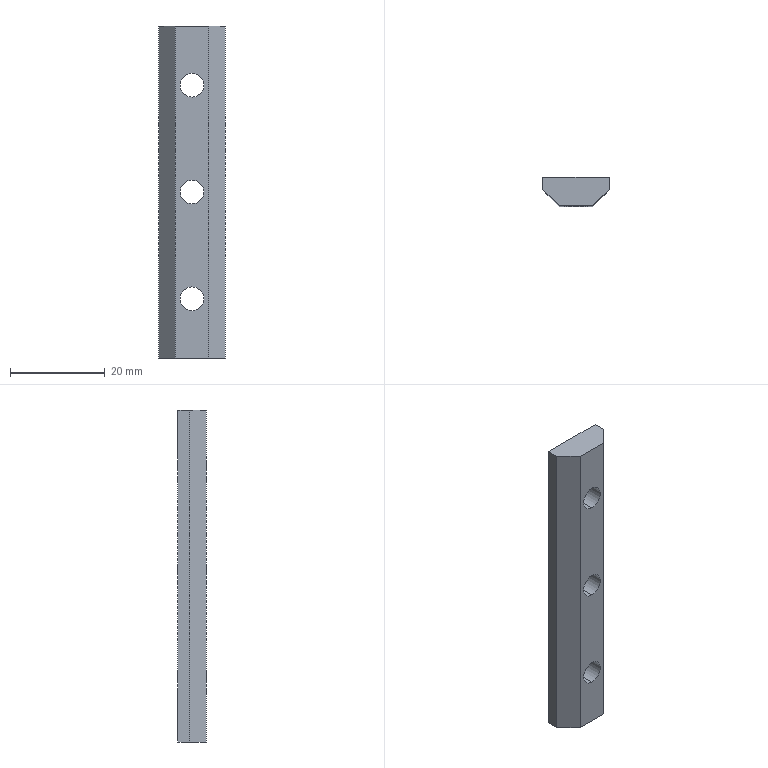Part | SolidWorks | features BaseBody 1 | 1 solid | 14 faces | box 14 x 6 x 70 mm | volume 4669 mm3 | plane 8 | cylinder 6 | commonest cylinder face diameters 5 x6
STEP:
#1=CARTESIAN_POINT('',(0.,-6.,-25.));
#2=VERTEX_POINT('',#1);
#3=CARTESIAN_POINT('',(0.,-6.,-20.));
#4=VERTEX_POINT('',#3);
#5=CARTESIAN_POINT('',(0.,-6.,-22.5));
#6=DIRECTION('',(0.,1.,0.));
#7=DIRECTION('',(-1.,0.,0.));
#8=AXIS2_PLACEMENT_3D('',#5,#6,#7);
#9=CIRCLE('',#8,2.5);
#10=EDGE_CURVE('',#2,#4,#9,.T.);
#11=ORIENTED_EDGE('',*,*,#10,.F.);
#12=CARTESIAN_POINT('',(0.,0.,-25.));
#13=VERTEX_POINT('',#12);
#14=CARTESIAN_POINT('',(0.,0.,-25.));
#15=DIRECTION('',(0.,1.,0.));
#16=VECTOR('',#15,1000.);
#17=LINE('',#14,#16);
#18=EDGE_CURVE('',#2,#13,#17,.T.);
#19=ORIENTED_EDGE('',*,*,#18,.T.);
#20=CARTESIAN_POINT('',(0.,0.,-20.));
#21=VERTEX_POINT('',#20);
#22=CARTESIAN_POINT('',(0.,0.,-22.5));
#23=DIRECTION('',(0.,1.,0.));
#24=DIRECTION('',(0.,0.,1.));
#25=AXIS2_PLACEMENT_3D('',#22,#23,#24);
#26=CIRCLE('',#25,2.5);
#27=EDGE_CURVE('',#13,#21,#26,.T.);
#28=ORIENTED_EDGE('',*,*,#27,.T.);
#29=CARTESIAN_POINT('',(0.,0.,-20.));
#30=DIRECTION('',(0.,1.,0.));
#31=VECTOR('',#30,1000.);
#32=LINE('',#29,#31);
#33=EDGE_CURVE('',#4,#21,#32,.T.);
#34=ORIENTED_EDGE('',*,*,#33,.F.);
#35=EDGE_LOOP('',(#11,#19,#28,#34));
#36=FACE_OUTER_BOUND('',#35,.T.);
#37=CARTESIAN_POINT('',(0.,0.,-22.5));
#38=DIRECTION('',(0.,1.,0.));
#39=DIRECTION('',(0.,0.,1.));
#40=AXIS2_PLACEMENT_3D('',#37,#38,#39);
#41=CYLINDRICAL_SURFACE('',#40,2.5);
#42=ADVANCED_FACE('',(#36),#41,.F.);
#43=CARTESIAN_POINT('',(0.,-6.,20.));
#44=VERTEX_POINT('',#43);
#45=CARTESIAN_POINT('',(0.,-6.,25.));
#46=VERTEX_POINT('',#45);
#47=CARTESIAN_POINT('',(0.,-6.,22.5));
#48=DIRECTION('',(0.,1.,0.));
#49=DIRECTION('',(-1.,0.,0.));
#50=AXIS2_PLACEMENT_3D('',#47,#48,#49);
#51=CIRCLE('',#50,2.5);
#52=EDGE_CURVE('',#44,#46,#51,.T.);
#53=ORIENTED_EDGE('',*,*,#52,.F.);
#54=CARTESIAN_POINT('',(0.,0.,20.));
#55=VERTEX_POINT('',#54);
#56=CARTESIAN_POINT('',(0.,0.,20.));
#57=DIRECTION('',(0.,1.,0.));
#58=VECTOR('',#57,1000.);
#59=LINE('',#56,#58);
#60=EDGE_CURVE('',#44,#55,#59,.T.);
#61=ORIENTED_EDGE('',*,*,#60,.T.);
#62=CARTESIAN_POINT('',(0.,0.,25.));
#63=VERTEX_POINT('',#62);
#64=CARTESIAN_POINT('',(0.,0.,22.5));
#65=DIRECTION('',(0.,1.,0.));
#66=DIRECTION('',(0.,0.,1.));
#67=AXIS2_PLACEMENT_3D('',#64,#65,#66);
#68=CIRCLE('',#67,2.5);
#69=EDGE_CURVE('',#55,#63,#68,.T.);
#70=ORIENTED_EDGE('',*,*,#69,.T.);
#71=CARTESIAN_POINT('',(0.,0.,25.));
#72=DIRECTION('',(0.,1.,0.));
#73=VECTOR('',#72,1000.);
#74=LINE('',#71,#73);
#75=EDGE_CURVE('',#46,#63,#74,.T.);
#76=ORIENTED_EDGE('',*,*,#75,.F.);
#77=EDGE_LOOP('',(#53,#61,#70,#76));
#78=FACE_OUTER_BOUND('',#77,.T.);
#79=CARTESIAN_POINT('',(0.,0.,22.5));
#80=DIRECTION('',(0.,1.,0.));
#81=DIRECTION('',(0.,0.,1.));
#82=AXIS2_PLACEMENT_3D('',#79,#80,#81);
#83=CYLINDRICAL_SURFACE('',#82,2.5);
#84=ADVANCED_FACE('',(#78),#83,.F.);
#85=CARTESIAN_POINT('',(0.,-6.,-2.5));
#86=VERTEX_POINT('',#85);
#87=CARTESIAN_POINT('',(0.,-6.,2.5));
#88=VERTEX_POINT('',#87);
#89=CARTESIAN_POINT('',(0.,-6.,0.));
#90=DIRECTION('',(0.,1.,0.));
#91=DIRECTION('',(-1.,0.,0.));
#92=AXIS2_PLACEMENT_3D('',#89,#90,#91);
#93=CIRCLE('',#92,2.5);
#94=EDGE_CURVE('',#86,#88,#93,.T.);
#95=ORIENTED_EDGE('',*,*,#94,.F.);
#96=CARTESIAN_POINT('',(0.,0.,-2.5));
#97=VERTEX_POINT('',#96);
#98=CARTESIAN_POINT('',(0.,0.,-2.5));
#99=DIRECTION('',(0.,1.,0.));
#100=VECTOR('',#99,1000.);
#101=LINE('',#98,#100);
#102=EDGE_CURVE('',#86,#97,#101,.T.);
#103=ORIENTED_EDGE('',*,*,#102,.T.);
#104=CARTESIAN_POINT('',(0.,0.,2.5));
#105=VERTEX_POINT('',#104);
#106=CARTESIAN_POINT('',(0.,0.,0.));
#107=DIRECTION('',(0.,1.,0.));
#108=DIRECTION('',(0.,0.,1.));
#109=AXIS2_PLACEMENT_3D('',#106,#107,#108);
#110=CIRCLE('',#109,2.5);
#111=EDGE_CURVE('',#97,#105,#110,.T.);
#112=ORIENTED_EDGE('',*,*,#111,.T.);
#113=CARTESIAN_POINT('',(0.,0.,2.5));
#114=DIRECTION('',(0.,1.,0.));
#115=VECTOR('',#114,1000.);
#116=LINE('',#113,#115);
#117=EDGE_CURVE('',#88,#105,#116,.T.);
#118=ORIENTED_EDGE('',*,*,#117,.F.);
#119=EDGE_LOOP('',(#95,#103,#112,#118));
#120=FACE_OUTER_BOUND('',#119,.T.);
#121=CARTESIAN_POINT('',(0.,0.,0.));
#122=DIRECTION('',(0.,1.,0.));
#123=DIRECTION('',(0.,0.,1.));
#124=AXIS2_PLACEMENT_3D('',#121,#122,#123);
#125=CYLINDRICAL_SURFACE('',#124,2.5);
#126=ADVANCED_FACE('',(#120),#125,.F.);
#127=CARTESIAN_POINT('',(-7.,0.,-35.));
#128=VERTEX_POINT('',#127);
#129=CARTESIAN_POINT('',(-7.,-2.5,-35.));
#130=VERTEX_POINT('',#129);
#131=CARTESIAN_POINT('',(-7.,-2.5,-35.));
#132=DIRECTION('',(0.,-1.,0.));
#133=VECTOR('',#132,1000.);
#134=LINE('',#131,#133);
#135=EDGE_CURVE('',#128,#130,#134,.T.);
#136=ORIENTED_EDGE('',*,*,#135,.F.);
#137=CARTESIAN_POINT('',(7.,0.,-35.));
#138=VERTEX_POINT('',#137);
#139=CARTESIAN_POINT('',(-7.,0.,-35.));
#140=DIRECTION('',(-1.,0.,0.));
#141=VECTOR('',#140,1000.);
#142=LINE('',#139,#141);
#143=EDGE_CURVE('',#138,#128,#142,.T.);
#144=ORIENTED_EDGE('',*,*,#143,.F.);
#145=CARTESIAN_POINT('',(7.,-2.5,-35.));
#146=VERTEX_POINT('',#145);
#147=CARTESIAN_POINT('',(7.,0.,-35.));
#148=DIRECTION('',(0.,1.,0.));
#149=VECTOR('',#148,1000.);
#150=LINE('',#147,#149);
#151=EDGE_CURVE('',#146,#138,#150,.T.);
#152=ORIENTED_EDGE('',*,*,#151,.F.);
#153=CARTESIAN_POINT('',(3.5,-6.,-35.));
#154=VERTEX_POINT('',#153);
#155=CARTESIAN_POINT('',(7.,-2.5,-35.));
#156=DIRECTION('',(0.7071,0.7071,0.));
#157=VECTOR('',#156,1000.);
#158=LINE('',#155,#157);
#159=EDGE_CURVE('',#154,#146,#158,.T.);
#160=ORIENTED_EDGE('',*,*,#159,.F.);
#161=CARTESIAN_POINT('',(-3.5,-6.,-35.));
#162=VERTEX_POINT('',#161);
#163=CARTESIAN_POINT('',(3.5,-6.,-35.));
#164=DIRECTION('',(1.,0.,0.));
#165=VECTOR('',#164,1000.);
#166=LINE('',#163,#165);
#167=EDGE_CURVE('',#162,#154,#166,.T.);
#168=ORIENTED_EDGE('',*,*,#167,.F.);
#169=CARTESIAN_POINT('',(-3.5,-6.,-35.));
#170=DIRECTION('',(0.7071,-0.7071,0.));
#171=VECTOR('',#170,1000.);
#172=LINE('',#169,#171);
#173=EDGE_CURVE('',#130,#162,#172,.T.);
#174=ORIENTED_EDGE('',*,*,#173,.F.);
#175=EDGE_LOOP('',(#136,#144,#152,#160,#168,#174));
#176=FACE_OUTER_BOUND('',#175,.T.);
#177=CARTESIAN_POINT('',(0.,0.,-35.));
#178=DIRECTION('',(0.,0.,-1.));
#179=DIRECTION('',(0.,-1.,0.));
#180=AXIS2_PLACEMENT_3D('',#177,#178,#179);
#181=PLANE('',#180);
#182=ADVANCED_FACE('',(#176),#181,.T.);
#183=CARTESIAN_POINT('',(-7.,0.,35.));
#184=VERTEX_POINT('',#183);
#185=CARTESIAN_POINT('',(-7.,-2.5,35.));
#186=VERTEX_POINT('',#185);
#187=CARTESIAN_POINT('',(-7.,-2.5,35.));
#188=DIRECTION('',(0.,-1.,0.));
#189=VECTOR('',#188,1000.);
#190=LINE('',#187,#189);
#191=EDGE_CURVE('',#184,#186,#190,.T.);
#192=ORIENTED_EDGE('',*,*,#191,.T.);
#193=CARTESIAN_POINT('',(-3.5,-6.,35.));
#194=VERTEX_POINT('',#193);
#195=CARTESIAN_POINT('',(-3.5,-6.,35.));
#196=DIRECTION('',(0.7071,-0.7071,0.));
#197=VECTOR('',#196,1000.);
#198=LINE('',#195,#197);
#199=EDGE_CURVE('',#186,#194,#198,.T.);
#200=ORIENTED_EDGE('',*,*,#199,.T.);
#201=CARTESIAN_POINT('',(3.5,-6.,35.));
#202=VERTEX_POINT('',#201);
#203=CARTESIAN_POINT('',(3.5,-6.,35.));
#204=DIRECTION('',(1.,0.,0.));
#205=VECTOR('',#204,1000.);
#206=LINE('',#203,#205);
#207=EDGE_CURVE('',#194,#202,#206,.T.);
#208=ORIENTED_EDGE('',*,*,#207,.T.);
#209=CARTESIAN_POINT('',(7.,-2.5,35.));
#210=VERTEX_POINT('',#209);
#211=CARTESIAN_POINT('',(7.,-2.5,35.));
#212=DIRECTION('',(0.7071,0.7071,0.));
#213=VECTOR('',#212,1000.);
#214=LINE('',#211,#213);
#215=EDGE_CURVE('',#202,#210,#214,.T.);
#216=ORIENTED_EDGE('',*,*,#215,.T.);
#217=CARTESIAN_POINT('',(7.,0.,35.));
#218=VERTEX_POINT('',#217);
#219=CARTESIAN_POINT('',(7.,0.,35.));
#220=DIRECTION('',(0.,1.,0.));
#221=VECTOR('',#220,1000.);
#222=LINE('',#219,#221);
#223=EDGE_CURVE('',#210,#218,#222,.T.);
#224=ORIENTED_EDGE('',*,*,#223,.T.);
#225=CARTESIAN_POINT('',(-7.,0.,35.));
#226=DIRECTION('',(-1.,0.,0.));
#227=VECTOR('',#226,1000.);
#228=LINE('',#225,#227);
#229=EDGE_CURVE('',#218,#184,#228,.T.);
#230=ORIENTED_EDGE('',*,*,#229,.T.);
#231=EDGE_LOOP('',(#192,#200,#208,#216,#224,#230));
#232=FACE_OUTER_BOUND('',#231,.T.);
#233=CARTESIAN_POINT('',(0.,0.,35.));
#234=DIRECTION('',(0.,0.,-1.));
#235=DIRECTION('',(0.,-1.,0.));
#236=AXIS2_PLACEMENT_3D('',#233,#234,#235);
#237=PLANE('',#236);
#238=ADVANCED_FACE('',(#232),#237,.F.);
#239=ORIENTED_EDGE('',*,*,#151,.T.);
#240=CARTESIAN_POINT('',(7.,0.,35.));
#241=DIRECTION('',(0.,0.,-1.));
#242=VECTOR('',#241,1000.);
#243=LINE('',#240,#242);
#244=EDGE_CURVE('',#218,#138,#243,.T.);
#245=ORIENTED_EDGE('',*,*,#244,.F.);
#246=ORIENTED_EDGE('',*,*,#223,.F.);
#247=CARTESIAN_POINT('',(7.,-2.5,35.));
#248=DIRECTION('',(0.,0.,-1.));
#249=VECTOR('',#248,1000.);
#250=LINE('',#247,#249);
#251=EDGE_CURVE('',#210,#146,#250,.T.);
#252=ORIENTED_EDGE('',*,*,#251,.T.);
#253=EDGE_LOOP('',(#239,#245,#246,#252));
#254=FACE_OUTER_BOUND('',#253,.T.);
#255=CARTESIAN_POINT('',(7.,0.,35.));
#256=DIRECTION('',(-1.,0.,0.));
#257=DIRECTION('',(0.,0.,1.));
#258=AXIS2_PLACEMENT_3D('',#255,#256,#257);
#259=PLANE('',#258);
#260=ADVANCED_FACE('',(#254),#259,.F.);
#261=ORIENTED_EDGE('',*,*,#159,.T.);
#262=ORIENTED_EDGE('',*,*,#251,.F.);
#263=ORIENTED_EDGE('',*,*,#215,.F.);
#264=CARTESIAN_POINT('',(3.5,-6.,35.));
#265=DIRECTION('',(0.,0.,-1.));
#266=VECTOR('',#265,1000.);
#267=LINE('',#264,#266);
#268=EDGE_CURVE('',#202,#154,#267,.T.);
#269=ORIENTED_EDGE('',*,*,#268,.T.);
#270=EDGE_LOOP('',(#261,#262,#263,#269));
#271=FACE_OUTER_BOUND('',#270,.T.);
#272=CARTESIAN_POINT('',(7.,-2.5,35.));
#273=DIRECTION('',(-0.7071,0.7071,0.));
#274=DIRECTION('',(0.,0.,1.));
#275=AXIS2_PLACEMENT_3D('',#272,#273,#274);
#276=PLANE('',#275);
#277=ADVANCED_FACE('',(#271),#276,.F.);
#278=CARTESIAN_POINT('',(0.,-6.,0.));
#279=DIRECTION('',(0.,1.,0.));
#280=DIRECTION('',(-1.,0.,0.));
#281=AXIS2_PLACEMENT_3D('',#278,#279,#280);
#282=CIRCLE('',#281,2.5);
#283=EDGE_CURVE('',#88,#86,#282,.T.);
#284=ORIENTED_EDGE('',*,*,#283,.T.);
#285=ORIENTED_EDGE('',*,*,#94,.T.);
#286=EDGE_LOOP('',(#284,#285));
#287=FACE_BOUND('',#286,.T.);
#288=CARTESIAN_POINT('',(0.,-6.,22.5));
#289=DIRECTION('',(0.,1.,0.));
#290=DIRECTION('',(-1.,0.,0.));
#291=AXIS2_PLACEMENT_3D('',#288,#289,#290);
#292=CIRCLE('',#291,2.5);
#293=EDGE_CURVE('',#46,#44,#292,.T.);
#294=ORIENTED_EDGE('',*,*,#293,.T.);
#295=ORIENTED_EDGE('',*,*,#52,.T.);
#296=EDGE_LOOP('',(#294,#295));
#297=FACE_BOUND('',#296,.T.);
#298=CARTESIAN_POINT('',(0.,-6.,-22.5));
#299=DIRECTION('',(0.,1.,0.));
#300=DIRECTION('',(-1.,0.,0.));
#301=AXIS2_PLACEMENT_3D('',#298,#299,#300);
#302=CIRCLE('',#301,2.5);
#303=EDGE_CURVE('',#4,#2,#302,.T.);
#304=ORIENTED_EDGE('',*,*,#303,.T.);
#305=ORIENTED_EDGE('',*,*,#10,.T.);
#306=EDGE_LOOP('',(#304,#305));
#307=FACE_BOUND('',#306,.T.);
#308=ORIENTED_EDGE('',*,*,#167,.T.);
#309=ORIENTED_EDGE('',*,*,#268,.F.);
#310=ORIENTED_EDGE('',*,*,#207,.F.);
#311=CARTESIAN_POINT('',(-3.5,-6.,35.));
#312=DIRECTION('',(0.,0.,-1.));
#313=VECTOR('',#312,1000.);
#314=LINE('',#311,#313);
#315=EDGE_CURVE('',#194,#162,#314,.T.);
#316=ORIENTED_EDGE('',*,*,#315,.T.);
#317=EDGE_LOOP('',(#308,#309,#310,#316));
#318=FACE_OUTER_BOUND('',#317,.T.);
#319=CARTESIAN_POINT('',(3.5,-6.,35.));
#320=DIRECTION('',(0.,1.,0.));
#321=DIRECTION('',(1.,0.,0.));
#322=AXIS2_PLACEMENT_3D('',#319,#320,#321);
#323=PLANE('',#322);
#324=ADVANCED_FACE('',(#287,#297,#307,#318),#323,.F.);
#325=ORIENTED_EDGE('',*,*,#173,.T.);
#326=ORIENTED_EDGE('',*,*,#315,.F.);
#327=ORIENTED_EDGE('',*,*,#199,.F.);
#328=CARTESIAN_POINT('',(-7.,-2.5,35.));
#329=DIRECTION('',(0.,0.,-1.));
#330=VECTOR('',#329,1000.);
#331=LINE('',#328,#330);
#332=EDGE_CURVE('',#186,#130,#331,.T.);
#333=ORIENTED_EDGE('',*,*,#332,.T.);
#334=EDGE_LOOP('',(#325,#326,#327,#333));
#335=FACE_OUTER_BOUND('',#334,.T.);
#336=CARTESIAN_POINT('',(-3.5,-6.,35.));
#337=DIRECTION('',(0.7071,0.7071,0.));
#338=DIRECTION('',(0.,0.,-1.));
#339=AXIS2_PLACEMENT_3D('',#336,#337,#338);
#340=PLANE('',#339);
#341=ADVANCED_FACE('',(#335),#340,.F.);
#342=ORIENTED_EDGE('',*,*,#135,.T.);
#343=ORIENTED_EDGE('',*,*,#332,.F.);
#344=ORIENTED_EDGE('',*,*,#191,.F.);
#345=CARTESIAN_POINT('',(-7.,0.,35.));
#346=DIRECTION('',(0.,0.,-1.));
#347=VECTOR('',#346,1000.);
#348=LINE('',#345,#347);
#349=EDGE_CURVE('',#184,#128,#348,.T.);
#350=ORIENTED_EDGE('',*,*,#349,.T.);
#351=EDGE_LOOP('',(#342,#343,#344,#350));
#352=FACE_OUTER_BOUND('',#351,.T.);
#353=CARTESIAN_POINT('',(-7.,-2.5,35.));
#354=DIRECTION('',(1.,0.,0.));
#355=DIRECTION('',(0.,1.,0.));
#356=AXIS2_PLACEMENT_3D('',#353,#354,#355);
#357=PLANE('',#356);
#358=ADVANCED_FACE('',(#352),#357,.F.);
#359=CARTESIAN_POINT('',(0.,0.,22.5));
#360=DIRECTION('',(0.,1.,0.));
#361=DIRECTION('',(0.,0.,1.));
#362=AXIS2_PLACEMENT_3D('',#359,#360,#361);
#363=CIRCLE('',#362,2.5);
#364=EDGE_CURVE('',#63,#55,#363,.T.);
#365=ORIENTED_EDGE('',*,*,#364,.F.);
#366=ORIENTED_EDGE('',*,*,#69,.F.);
#367=EDGE_LOOP('',(#365,#366));
#368=FACE_BOUND('',#367,.T.);
#369=CARTESIAN_POINT('',(0.,0.,0.));
#370=DIRECTION('',(0.,1.,0.));
#371=DIRECTION('',(0.,0.,1.));
#372=AXIS2_PLACEMENT_3D('',#369,#370,#371);
#373=CIRCLE('',#372,2.5);
#374=EDGE_CURVE('',#105,#97,#373,.T.);
#375=ORIENTED_EDGE('',*,*,#374,.F.);
#376=ORIENTED_EDGE('',*,*,#111,.F.);
#377=EDGE_LOOP('',(#375,#376));
#378=FACE_BOUND('',#377,.T.);
#379=CARTESIAN_POINT('',(0.,0.,-22.5));
#380=DIRECTION('',(0.,1.,0.));
#381=DIRECTION('',(0.,0.,1.));
#382=AXIS2_PLACEMENT_3D('',#379,#380,#381);
#383=CIRCLE('',#382,2.5);
#384=EDGE_CURVE('',#21,#13,#383,.T.);
#385=ORIENTED_EDGE('',*,*,#384,.F.);
#386=ORIENTED_EDGE('',*,*,#27,.F.);
#387=EDGE_LOOP('',(#385,#386));
#388=FACE_BOUND('',#387,.T.);
#389=ORIENTED_EDGE('',*,*,#143,.T.);
#390=ORIENTED_EDGE('',*,*,#349,.F.);
#391=ORIENTED_EDGE('',*,*,#229,.F.);
#392=ORIENTED_EDGE('',*,*,#244,.T.);
#393=EDGE_LOOP('',(#389,#390,#391,#392));
#394=FACE_OUTER_BOUND('',#393,.T.);
#395=CARTESIAN_POINT('',(-7.,0.,35.));
#396=DIRECTION('',(0.,-1.,0.));
#397=DIRECTION('',(0.,0.,-1.));
#398=AXIS2_PLACEMENT_3D('',#395,#396,#397);
#399=PLANE('',#398);
#400=ADVANCED_FACE('',(#368,#378,#388,#394),#399,.F.);
#401=ORIENTED_EDGE('',*,*,#102,.F.);
#402=ORIENTED_EDGE('',*,*,#283,.F.);
#403=ORIENTED_EDGE('',*,*,#117,.T.);
#404=ORIENTED_EDGE('',*,*,#374,.T.);
#405=EDGE_LOOP('',(#401,#402,#403,#404));
#406=FACE_OUTER_BOUND('',#405,.T.);
#407=CARTESIAN_POINT('',(0.,0.,0.));
#408=DIRECTION('',(0.,1.,0.));
#409=DIRECTION('',(0.,0.,1.));
#410=AXIS2_PLACEMENT_3D('',#407,#408,#409);
#411=CYLINDRICAL_SURFACE('',#410,2.5);
#412=ADVANCED_FACE('',(#406),#411,.F.);
#413=ORIENTED_EDGE('',*,*,#60,.F.);
#414=ORIENTED_EDGE('',*,*,#293,.F.);
#415=ORIENTED_EDGE('',*,*,#75,.T.);
#416=ORIENTED_EDGE('',*,*,#364,.T.);
#417=EDGE_LOOP('',(#413,#414,#415,#416));
#418=FACE_OUTER_BOUND('',#417,.T.);
#419=CARTESIAN_POINT('',(0.,0.,22.5));
#420=DIRECTION('',(0.,1.,0.));
#421=DIRECTION('',(0.,0.,1.));
#422=AXIS2_PLACEMENT_3D('',#419,#420,#421);
#423=CYLINDRICAL_SURFACE('',#422,2.5);
#424=ADVANCED_FACE('',(#418),#423,.F.);
#425=ORIENTED_EDGE('',*,*,#18,.F.);
#426=ORIENTED_EDGE('',*,*,#303,.F.);
#427=ORIENTED_EDGE('',*,*,#33,.T.);
#428=ORIENTED_EDGE('',*,*,#384,.T.);
#429=EDGE_LOOP('',(#425,#426,#427,#428));
#430=FACE_OUTER_BOUND('',#429,.T.);
#431=CARTESIAN_POINT('',(0.,0.,-22.5));
#432=DIRECTION('',(0.,1.,0.));
#433=DIRECTION('',(0.,0.,1.));
#434=AXIS2_PLACEMENT_3D('',#431,#432,#433);
#435=CYLINDRICAL_SURFACE('',#434,2.5);
#436=ADVANCED_FACE('',(#430),#435,.F.);
#437=CLOSED_SHELL('',(#42,#84,#126,#182,#238,#260,#277,#324,#341,#358,#400,#412,#424,#436));
#438=MANIFOLD_SOLID_BREP('',#437);
#439=CARTESIAN_POINT('',(0.,0.,0.));
#440=DIRECTION('',(0.,0.,1.));
#441=DIRECTION('',(1.,0.,0.));
#442=AXIS2_PLACEMENT_3D('',#439,#440,#441);
#443=(LENGTH_UNIT()NAMED_UNIT(*)SI_UNIT(.MILLI.,.METRE.));
#444=UNCERTAINTY_MEASURE_WITH_UNIT(LENGTH_MEASURE(0.00001),#443,'','');
#445=(NAMED_UNIT(*)PLANE_ANGLE_UNIT()SI_UNIT($,.RADIAN.));
#446=(NAMED_UNIT(*)SI_UNIT($,.STERADIAN.)SOLID_ANGLE_UNIT());
#447=(GEOMETRIC_REPRESENTATION_CONTEXT(3)GLOBAL_UNCERTAINTY_ASSIGNED_CONTEXT((#444))GLOBAL_UNIT_ASSIGNED_CONTEXT((#443,#445,#446))REPRESENTATION_CONTEXT('',''));
#448=ADVANCED_BREP_SHAPE_REPRESENTATION('',(#438,#442),#447);